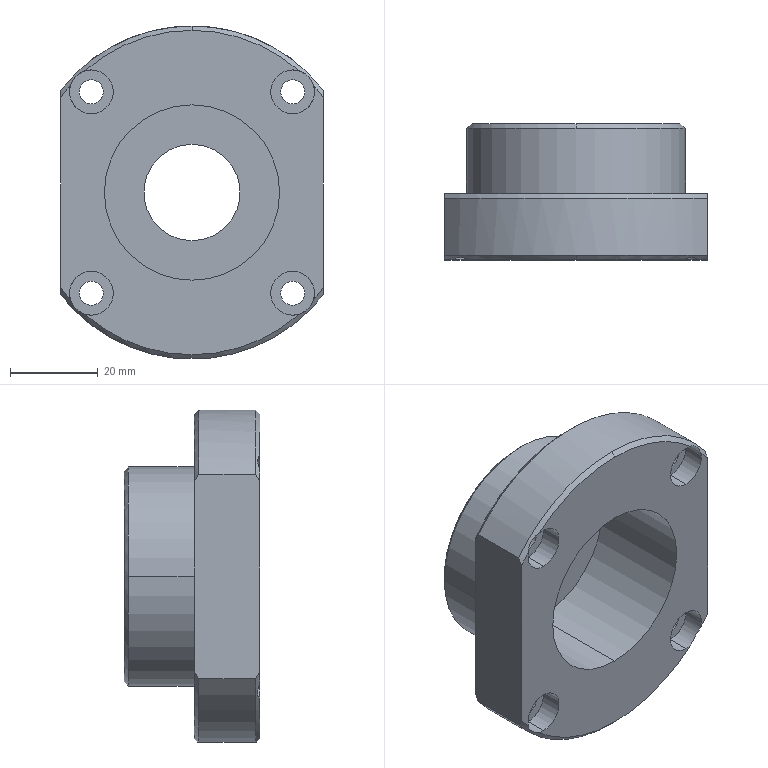Part | STEP file | fBY02F02M-00-25A | 1 solid | 44 faces | box 60 x 31 x 75.753 mm | volume 56251 mm3 | cylinder 25 | plane 11 | cone 8 | commonest cylinder face diameters 5.5 x8 10 x8 76 x3 22 x2 40 x2 50 x2